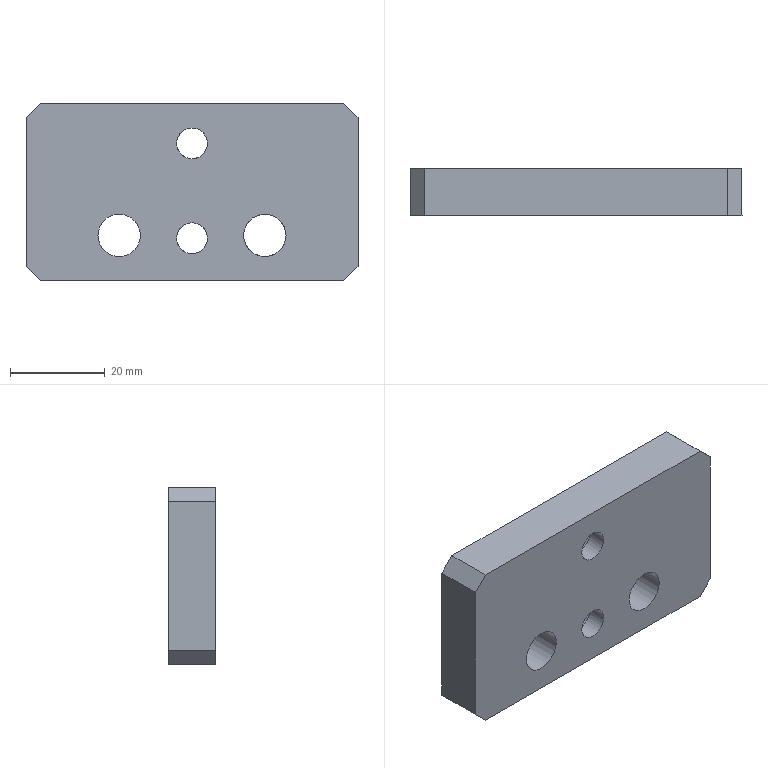Part | STEP file | 1_id1138_x_t | 1 solid | 18 faces | box 70 x 10 x 37.5 mm | volume 23507 mm3 | plane 12 | cylinder 6 | commonest cylinder face diameters 6.5 x2 8.95 x2 10.5 x2
STEP:
#1=CARTESIAN_POINT('',(0.,0.,0.));
#2=DIRECTION('',(0.,0.,1.));
#3=DIRECTION('',(1.,0.,0.));
#4=AXIS2_PLACEMENT_3D('',#1,#2,#3);
#5=CARTESIAN_POINT('',(750.075,188.975,-66.026));
#6=VERTEX_POINT('',#5);
#7=CARTESIAN_POINT('',(750.075,188.975,-71.276));
#8=DIRECTION('',(0.,1.,0.));
#9=DIRECTION('',(0.,0.,1.));
#10=AXIS2_PLACEMENT_3D('',#7,#8,#9);
#11=CIRCLE('',#10,5.25);
#12=CARTESIAN_POINT('',(750.075,188.975,-71.276));
#13=DIRECTION('',(0.,-1.,0.));
#14=DIRECTION('',(0.,0.,1.));
#15=AXIS2_PLACEMENT_3D('',#12,#13,#14);
#16=PLANE('',#15);
#17=CARTESIAN_POINT('',(5.25,0.));
#18=CARTESIAN_POINT('',(5.25,-9.093));
#19=CARTESIAN_POINT('',(-2.625,-4.547));
#20=CARTESIAN_POINT('',(-10.5,0.));
#21=CARTESIAN_POINT('',(-2.625,4.547));
#22=CARTESIAN_POINT('',(5.25,9.093));
#23=CARTESIAN_POINT('',(5.25,0.));
#24=(BOUNDED_CURVE()B_SPLINE_CURVE(2,(#17,#18,#19,#20,#21,#22,#23),.UNSPECIFIED.,.T.,.F.)B_SPLINE_CURVE_WITH_KNOTS((1,2,2,2,2,1),(-2.094,0.,2.094,4.189,6.283,8.378),.UNSPECIFIED.)CURVE()GEOMETRIC_REPRESENTATION_ITEM()RATIONAL_B_SPLINE_CURVE((1.,0.5,1.,0.5,1.,0.5,1.))REPRESENTATION_ITEM(''));
#25=(GEOMETRIC_REPRESENTATION_CONTEXT(2)PARAMETRIC_REPRESENTATION_CONTEXT()REPRESENTATION_CONTEXT('',''));
#26=DEFINITIONAL_REPRESENTATION('',(#24),#25);
#27=PCURVE('',#16,#26);
#28=CARTESIAN_POINT('',(750.075,194.975,-71.276));
#29=DIRECTION('',(0.,-1.,0.));
#30=DIRECTION('',(0.,0.,1.));
#31=AXIS2_PLACEMENT_3D('',#28,#29,#30);
#32=CYLINDRICAL_SURFACE('',#31,5.25);
#33=CARTESIAN_POINT('',(6.283,6.));
#34=DIRECTION('',(-1.,0.));
#35=VECTOR('',#34,1.);
#36=LINE('',#33,#35);
#37=(GEOMETRIC_REPRESENTATION_CONTEXT(2)PARAMETRIC_REPRESENTATION_CONTEXT()REPRESENTATION_CONTEXT('',''));
#38=DEFINITIONAL_REPRESENTATION('',(#36),#37);
#39=PCURVE('',#32,#38);
#40=SURFACE_CURVE('',#11,(#27,#39),.PCURVE_S1.);
#41=EDGE_CURVE('',#6,#6,#40,.T.);
#42=ORIENTED_EDGE('',*,*,#41,.T.);
#43=EDGE_LOOP('',(#42));
#44=FACE_BOUND('',#43,.T.);
#45=CARTESIAN_POINT('',(750.075,188.975,-74.526));
#46=VERTEX_POINT('',#45);
#47=CARTESIAN_POINT('',(750.075,188.975,-71.276));
#48=DIRECTION('',(0.,-1.,0.));
#49=DIRECTION('',(0.,0.,-1.));
#50=AXIS2_PLACEMENT_3D('',#47,#48,#49);
#51=CIRCLE('',#50,3.25);
#52=CARTESIAN_POINT('',(0.,-0.000000001));
#53=DIRECTION('',(-1.,0.));
#54=AXIS2_PLACEMENT_2D('',#52,#53);
#55=CIRCLE('',#54,3.25);
#56=(GEOMETRIC_REPRESENTATION_CONTEXT(2)PARAMETRIC_REPRESENTATION_CONTEXT()REPRESENTATION_CONTEXT('',''));
#57=DEFINITIONAL_REPRESENTATION('',(#55),#56);
#58=PCURVE('',#16,#57);
#59=CARTESIAN_POINT('',(750.075,185.725,-71.276));
#60=DIRECTION('',(0.,-1.,0.));
#61=DIRECTION('',(-1.,0.,0.));
#62=AXIS2_PLACEMENT_3D('',#59,#60,#61);
#63=CYLINDRICAL_SURFACE('',#62,3.25);
#64=CARTESIAN_POINT('',(1.571,-3.25));
#65=DIRECTION('',(1.,0.));
#66=VECTOR('',#65,1.);
#67=LINE('',#64,#66);
#68=(GEOMETRIC_REPRESENTATION_CONTEXT(2)PARAMETRIC_REPRESENTATION_CONTEXT()REPRESENTATION_CONTEXT('',''));
#69=DEFINITIONAL_REPRESENTATION('',(#67),#68);
#70=PCURVE('',#63,#69);
#71=SURFACE_CURVE('',#51,(#58,#70),.PCURVE_S1.);
#72=EDGE_CURVE('',#46,#46,#71,.T.);
#73=ORIENTED_EDGE('',*,*,#72,.T.);
#74=EDGE_LOOP('',(#73));
#75=FACE_BOUND('',#74,.T.);
#76=ADVANCED_FACE('',(#44,#75),#16,.F.);
#77=ORIENTED_EDGE('',*,*,#41,.T.);
#78=CARTESIAN_POINT('',(750.075,194.975,-66.026));
#79=VERTEX_POINT('',#78);
#80=CARTESIAN_POINT('',(750.075,194.975,-66.026));
#81=CARTESIAN_POINT('',(750.075,188.975,-66.026));
#82=B_SPLINE_CURVE_WITH_KNOTS('',1,(#80,#81),.UNSPECIFIED.,.F.,.F.,(2,2),(-0.000000002,6.),.PIECEWISE_BEZIER_KNOTS.);
#83=CARTESIAN_POINT('',(0.,0.));
#84=DIRECTION('',(0.,1.));
#85=VECTOR('',#84,1.);
#86=LINE('',#83,#85);
#87=(GEOMETRIC_REPRESENTATION_CONTEXT(2)PARAMETRIC_REPRESENTATION_CONTEXT()REPRESENTATION_CONTEXT('',''));
#88=DEFINITIONAL_REPRESENTATION('',(#86),#87);
#89=PCURVE('',#32,#88);
#90=CARTESIAN_POINT('',(6.283,0.));
#91=DIRECTION('',(0.,1.));
#92=VECTOR('',#91,1.);
#93=LINE('',#90,#92);
#94=(GEOMETRIC_REPRESENTATION_CONTEXT(2)PARAMETRIC_REPRESENTATION_CONTEXT()REPRESENTATION_CONTEXT('',''));
#95=DEFINITIONAL_REPRESENTATION('',(#93),#94);
#96=PCURVE('',#32,#95);
#97=SEAM_CURVE('',#82,(#89,#96),.PCURVE_S1.);
#98=EDGE_CURVE('',#79,#6,#97,.T.);
#99=ORIENTED_EDGE('',*,*,#98,.F.);
#100=CARTESIAN_POINT('',(750.075,194.975,-76.526));
#101=VERTEX_POINT('',#100);
#102=CARTESIAN_POINT('',(750.075,194.975,-71.276));
#103=DIRECTION('',(0.,-1.,0.));
#104=DIRECTION('',(0.,0.,-1.));
#105=AXIS2_PLACEMENT_3D('',#102,#103,#104);
#106=CIRCLE('',#105,5.25);
#107=CARTESIAN_POINT('',(-3.142,-0.000000002));
#108=DIRECTION('',(1.,0.));
#109=VECTOR('',#108,1.);
#110=LINE('',#107,#109);
#111=(GEOMETRIC_REPRESENTATION_CONTEXT(2)PARAMETRIC_REPRESENTATION_CONTEXT()REPRESENTATION_CONTEXT('',''));
#112=DEFINITIONAL_REPRESENTATION('',(#110),#111);
#113=PCURVE('',#32,#112);
#114=CARTESIAN_POINT('',(784.423,194.975,-37.776));
#115=DIRECTION('',(0.,1.,0.));
#116=DIRECTION('',(1.,0.,0.));
#117=AXIS2_PLACEMENT_3D('',#114,#115,#116);
#118=PLANE('',#117);
#119=CARTESIAN_POINT('',(-34.348,38.75));
#120=CARTESIAN_POINT('',(-25.254,38.75));
#121=CARTESIAN_POINT('',(-29.801,30.875));
#122=CARTESIAN_POINT('',(-34.348,23.));
#123=CARTESIAN_POINT('',(-38.894,30.875));
#124=CARTESIAN_POINT('',(-43.441,38.75));
#125=CARTESIAN_POINT('',(-34.348,38.75));
#126=(BOUNDED_CURVE()B_SPLINE_CURVE(2,(#119,#120,#121,#122,#123,#124,#125),.UNSPECIFIED.,.T.,.F.)B_SPLINE_CURVE_WITH_KNOTS((1,2,2,2,2,1),(-2.094,0.,2.094,4.189,6.283,8.378),.UNSPECIFIED.)CURVE()GEOMETRIC_REPRESENTATION_ITEM()RATIONAL_B_SPLINE_CURVE((1.,0.5,1.,0.5,1.,0.5,1.))REPRESENTATION_ITEM(''));
#127=(GEOMETRIC_REPRESENTATION_CONTEXT(2)PARAMETRIC_REPRESENTATION_CONTEXT()REPRESENTATION_CONTEXT('',''));
#128=DEFINITIONAL_REPRESENTATION('',(#126),#127);
#129=PCURVE('',#118,#128);
#130=SURFACE_CURVE('',#106,(#113,#129),.PCURVE_S1.);
#131=EDGE_CURVE('',#79,#101,#130,.T.);
#132=ORIENTED_EDGE('',*,*,#131,.T.);
#133=CARTESIAN_POINT('',(750.075,194.975,-71.276));
#134=DIRECTION('',(0.,-1.,0.));
#135=DIRECTION('',(0.,0.,-1.));
#136=AXIS2_PLACEMENT_3D('',#133,#134,#135);
#137=CIRCLE('',#136,5.25);
#138=CARTESIAN_POINT('',(3.142,-0.000000002));
#139=DIRECTION('',(1.,0.));
#140=VECTOR('',#139,1.);
#141=LINE('',#138,#140);
#142=(GEOMETRIC_REPRESENTATION_CONTEXT(2)PARAMETRIC_REPRESENTATION_CONTEXT()REPRESENTATION_CONTEXT('',''));
#143=DEFINITIONAL_REPRESENTATION('',(#141),#142);
#144=PCURVE('',#32,#143);
#145=CARTESIAN_POINT('',(-34.348,38.75));
#146=CARTESIAN_POINT('',(-25.254,38.75));
#147=CARTESIAN_POINT('',(-29.801,30.875));
#148=CARTESIAN_POINT('',(-34.348,23.));
#149=CARTESIAN_POINT('',(-38.894,30.875));
#150=CARTESIAN_POINT('',(-43.441,38.75));
#151=CARTESIAN_POINT('',(-34.348,38.75));
#152=(BOUNDED_CURVE()B_SPLINE_CURVE(2,(#145,#146,#147,#148,#149,#150,#151),.UNSPECIFIED.,.T.,.F.)B_SPLINE_CURVE_WITH_KNOTS((1,2,2,2,2,1),(-2.094,0.,2.094,4.189,6.283,8.378),.UNSPECIFIED.)CURVE()GEOMETRIC_REPRESENTATION_ITEM()RATIONAL_B_SPLINE_CURVE((1.,0.5,1.,0.5,1.,0.5,1.))REPRESENTATION_ITEM(''));
#153=(GEOMETRIC_REPRESENTATION_CONTEXT(2)PARAMETRIC_REPRESENTATION_CONTEXT()REPRESENTATION_CONTEXT('',''));
#154=DEFINITIONAL_REPRESENTATION('',(#152),#153);
#155=PCURVE('',#118,#154);
#156=SURFACE_CURVE('',#137,(#144,#155),.PCURVE_S1.);
#157=EDGE_CURVE('',#101,#79,#156,.T.);
#158=ORIENTED_EDGE('',*,*,#157,.T.);
#159=ORIENTED_EDGE('',*,*,#98,.T.);
#160=EDGE_LOOP('',(#77,#99,#132,#158,#159));
#161=FACE_BOUND('',#160,.F.);
#162=ADVANCED_FACE('',(#161),#32,.F.);
#163=CARTESIAN_POINT('',(785.075,194.975,-77.276));
#164=VERTEX_POINT('',#163);
#165=CARTESIAN_POINT('',(782.075,194.975,-80.276));
#166=VERTEX_POINT('',#165);
#167=CARTESIAN_POINT('',(785.075,194.975,-77.276));
#168=DIRECTION('',(-0.7071,0.,-0.7071));
#169=VECTOR('',#168,1.);
#170=LINE('',#167,#169);
#171=CARTESIAN_POINT('',(0.6524,39.5));
#172=DIRECTION('',(-0.7071,0.7071));
#173=VECTOR('',#172,1.);
#174=LINE('',#171,#173);
#175=(GEOMETRIC_REPRESENTATION_CONTEXT(2)PARAMETRIC_REPRESENTATION_CONTEXT()REPRESENTATION_CONTEXT('',''));
#176=DEFINITIONAL_REPRESENTATION('',(#174),#175);
#177=PCURVE('',#118,#176);
#178=CARTESIAN_POINT('',(782.075,183.425,-80.276));
#179=DIRECTION('',(-0.7071,0.,0.7071));
#180=DIRECTION('',(0.7071,0.,0.7071));
#181=AXIS2_PLACEMENT_3D('',#178,#179,#180);
#182=PLANE('',#181);
#183=CARTESIAN_POINT('',(4.243,11.55));
#184=DIRECTION('',(-1.,0.));
#185=VECTOR('',#184,1.);
#186=LINE('',#183,#185);
#187=(GEOMETRIC_REPRESENTATION_CONTEXT(2)PARAMETRIC_REPRESENTATION_CONTEXT()REPRESENTATION_CONTEXT('',''));
#188=DEFINITIONAL_REPRESENTATION('',(#186),#187);
#189=PCURVE('',#182,#188);
#190=SURFACE_CURVE('',#170,(#177,#189),.PCURVE_S1.);
#191=EDGE_CURVE('',#164,#166,#190,.T.);
#192=ORIENTED_EDGE('',*,*,#191,.T.);
#193=CARTESIAN_POINT('',(718.075,194.975,-80.276));
#194=VERTEX_POINT('',#193);
#195=CARTESIAN_POINT('',(718.075,194.975,-80.276));
#196=DIRECTION('',(1.,0.,0.));
#197=VECTOR('',#196,1.);
#198=LINE('',#195,#197);
#199=CARTESIAN_POINT('',(-66.348,42.5));
#200=DIRECTION('',(1.,0.));
#201=VECTOR('',#200,1.);
#202=LINE('',#199,#201);
#203=(GEOMETRIC_REPRESENTATION_CONTEXT(2)PARAMETRIC_REPRESENTATION_CONTEXT()REPRESENTATION_CONTEXT('',''));
#204=DEFINITIONAL_REPRESENTATION('',(#202),#203);
#205=PCURVE('',#118,#204);
#206=CARTESIAN_POINT('',(728.423,183.425,-80.276));
#207=DIRECTION('',(0.,0.,1.));
#208=DIRECTION('',(-1.,0.,0.));
#209=AXIS2_PLACEMENT_3D('',#206,#207,#208);
#210=PLANE('',#209);
#211=CARTESIAN_POINT('',(10.348,-11.55));
#212=DIRECTION('',(-1.,0.));
#213=VECTOR('',#212,1.);
#214=LINE('',#211,#213);
#215=(GEOMETRIC_REPRESENTATION_CONTEXT(2)PARAMETRIC_REPRESENTATION_CONTEXT()REPRESENTATION_CONTEXT('',''));
#216=DEFINITIONAL_REPRESENTATION('',(#214),#215);
#217=PCURVE('',#210,#216);
#218=SURFACE_CURVE('',#198,(#205,#217),.PCURVE_S1.);
#219=EDGE_CURVE('',#194,#166,#218,.T.);
#220=ORIENTED_EDGE('',*,*,#219,.F.);
#221=CARTESIAN_POINT('',(715.075,194.975,-77.276));
#222=VERTEX_POINT('',#221);
#223=CARTESIAN_POINT('',(718.075,194.975,-80.276));
#224=DIRECTION('',(-0.7071,0.,0.7071));
#225=VECTOR('',#224,1.);
#226=LINE('',#223,#225);
#227=CARTESIAN_POINT('',(-66.348,42.5));
#228=DIRECTION('',(-0.7071,-0.7071));
#229=VECTOR('',#228,1.);
#230=LINE('',#227,#229);
#231=(GEOMETRIC_REPRESENTATION_CONTEXT(2)PARAMETRIC_REPRESENTATION_CONTEXT()REPRESENTATION_CONTEXT('',''));
#232=DEFINITIONAL_REPRESENTATION('',(#230),#231);
#233=PCURVE('',#118,#232);
#234=CARTESIAN_POINT('',(718.075,183.425,-80.276));
#235=DIRECTION('',(0.7071,0.,0.7071));
#236=DIRECTION('',(0.7071,0.,-0.7071));
#237=AXIS2_PLACEMENT_3D('',#234,#235,#236);
#238=PLANE('',#237);
#239=CARTESIAN_POINT('',(0.,11.55));
#240=DIRECTION('',(-1.,0.));
#241=VECTOR('',#240,1.);
#242=LINE('',#239,#241);
#243=(GEOMETRIC_REPRESENTATION_CONTEXT(2)PARAMETRIC_REPRESENTATION_CONTEXT()REPRESENTATION_CONTEXT('',''));
#244=DEFINITIONAL_REPRESENTATION('',(#242),#243);
#245=PCURVE('',#238,#244);
#246=SURFACE_CURVE('',#226,(#233,#245),.PCURVE_S1.);
#247=EDGE_CURVE('',#194,#222,#246,.T.);
#248=ORIENTED_EDGE('',*,*,#247,.T.);
#249=CARTESIAN_POINT('',(715.075,194.975,-45.776));
#250=VERTEX_POINT('',#249);
#251=CARTESIAN_POINT('',(715.075,194.975,-77.276));
#252=DIRECTION('',(0.,0.,1.));
#253=VECTOR('',#252,1.);
#254=LINE('',#251,#253);
#255=CARTESIAN_POINT('',(-69.348,39.5));
#256=DIRECTION('',(0.,-1.));
#257=VECTOR('',#256,1.);
#258=LINE('',#255,#257);
#259=(GEOMETRIC_REPRESENTATION_CONTEXT(2)PARAMETRIC_REPRESENTATION_CONTEXT()REPRESENTATION_CONTEXT('',''));
#260=DEFINITIONAL_REPRESENTATION('',(#258),#259);
#261=PCURVE('',#118,#260);
#262=CARTESIAN_POINT('',(715.075,191.975,-61.526));
#263=DIRECTION('',(1.,0.,0.));
#264=DIRECTION('',(0.,0.,-1.));
#265=AXIS2_PLACEMENT_3D('',#262,#263,#264);
#266=PLANE('',#265);
#267=CARTESIAN_POINT('',(15.75,3.));
#268=DIRECTION('',(-1.,0.));
#269=VECTOR('',#268,1.);
#270=LINE('',#267,#269);
#271=(GEOMETRIC_REPRESENTATION_CONTEXT(2)PARAMETRIC_REPRESENTATION_CONTEXT()REPRESENTATION_CONTEXT('',''));
#272=DEFINITIONAL_REPRESENTATION('',(#270),#271);
#273=PCURVE('',#266,#272);
#274=SURFACE_CURVE('',#254,(#261,#273),.PCURVE_S1.);
#275=EDGE_CURVE('',#222,#250,#274,.T.);
#276=ORIENTED_EDGE('',*,*,#275,.T.);
#277=CARTESIAN_POINT('',(718.075,194.975,-42.776));
#278=VERTEX_POINT('',#277);
#279=CARTESIAN_POINT('',(715.075,194.975,-45.776));
#280=DIRECTION('',(0.7071,0.,0.7071));
#281=VECTOR('',#280,1.);
#282=LINE('',#279,#281);
#283=CARTESIAN_POINT('',(-69.348,8.));
#284=DIRECTION('',(0.7071,-0.7071));
#285=VECTOR('',#284,1.);
#286=LINE('',#283,#285);
#287=(GEOMETRIC_REPRESENTATION_CONTEXT(2)PARAMETRIC_REPRESENTATION_CONTEXT()REPRESENTATION_CONTEXT('',''));
#288=DEFINITIONAL_REPRESENTATION('',(#286),#287);
#289=PCURVE('',#118,#288);
#290=CARTESIAN_POINT('',(718.075,183.425,-42.776));
#291=DIRECTION('',(0.7071,0.,-0.7071));
#292=DIRECTION('',(-0.7071,0.,-0.7071));
#293=AXIS2_PLACEMENT_3D('',#290,#291,#292);
#294=PLANE('',#293);
#295=CARTESIAN_POINT('',(4.243,11.55));
#296=DIRECTION('',(-1.,0.));
#297=VECTOR('',#296,1.);
#298=LINE('',#295,#297);
#299=(GEOMETRIC_REPRESENTATION_CONTEXT(2)PARAMETRIC_REPRESENTATION_CONTEXT()REPRESENTATION_CONTEXT('',''));
#300=DEFINITIONAL_REPRESENTATION('',(#298),#299);
#301=PCURVE('',#294,#300);
#302=SURFACE_CURVE('',#282,(#289,#301),.PCURVE_S1.);
#303=EDGE_CURVE('',#250,#278,#302,.T.);
#304=ORIENTED_EDGE('',*,*,#303,.T.);
#305=CARTESIAN_POINT('',(782.075,194.975,-42.776));
#306=VERTEX_POINT('',#305);
#307=CARTESIAN_POINT('',(782.075,194.975,-42.776));
#308=DIRECTION('',(-1.,0.,0.));
#309=VECTOR('',#308,1.);
#310=LINE('',#307,#309);
#311=CARTESIAN_POINT('',(-2.348,5.));
#312=DIRECTION('',(-1.,0.));
#313=VECTOR('',#312,1.);
#314=LINE('',#311,#313);
#315=(GEOMETRIC_REPRESENTATION_CONTEXT(2)PARAMETRIC_REPRESENTATION_CONTEXT()REPRESENTATION_CONTEXT('',''));
#316=DEFINITIONAL_REPRESENTATION('',(#314),#315);
#317=PCURVE('',#118,#316);
#318=CARTESIAN_POINT('',(775.423,183.425,-42.776));
#319=DIRECTION('',(0.,0.,-1.));
#320=DIRECTION('',(0.,-1.,0.));
#321=AXIS2_PLACEMENT_3D('',#318,#319,#320);
#322=PLANE('',#321);
#323=CARTESIAN_POINT('',(-11.55,-6.652));
#324=DIRECTION('',(0.,1.));
#325=VECTOR('',#324,1.);
#326=LINE('',#323,#325);
#327=(GEOMETRIC_REPRESENTATION_CONTEXT(2)PARAMETRIC_REPRESENTATION_CONTEXT()REPRESENTATION_CONTEXT('',''));
#328=DEFINITIONAL_REPRESENTATION('',(#326),#327);
#329=PCURVE('',#322,#328);
#330=SURFACE_CURVE('',#310,(#317,#329),.PCURVE_S1.);
#331=EDGE_CURVE('',#306,#278,#330,.T.);
#332=ORIENTED_EDGE('',*,*,#331,.F.);
#333=CARTESIAN_POINT('',(785.075,194.975,-45.776));
#334=VERTEX_POINT('',#333);
#335=CARTESIAN_POINT('',(782.075,194.975,-42.776));
#336=DIRECTION('',(0.7071,0.,-0.7071));
#337=VECTOR('',#336,1.);
#338=LINE('',#335,#337);
#339=CARTESIAN_POINT('',(-2.348,5.));
#340=DIRECTION('',(0.7071,0.7071));
#341=VECTOR('',#340,1.);
#342=LINE('',#339,#341);
#343=(GEOMETRIC_REPRESENTATION_CONTEXT(2)PARAMETRIC_REPRESENTATION_CONTEXT()REPRESENTATION_CONTEXT('',''));
#344=DEFINITIONAL_REPRESENTATION('',(#342),#343);
#345=PCURVE('',#118,#344);
#346=CARTESIAN_POINT('',(782.075,183.425,-42.776));
#347=DIRECTION('',(-0.7071,0.,-0.7071));
#348=DIRECTION('',(-0.7071,0.,0.7071));
#349=AXIS2_PLACEMENT_3D('',#346,#347,#348);
#350=PLANE('',#349);
#351=CARTESIAN_POINT('',(0.,11.55));
#352=DIRECTION('',(-1.,0.));
#353=VECTOR('',#352,1.);
#354=LINE('',#351,#353);
#355=(GEOMETRIC_REPRESENTATION_CONTEXT(2)PARAMETRIC_REPRESENTATION_CONTEXT()REPRESENTATION_CONTEXT('',''));
#356=DEFINITIONAL_REPRESENTATION('',(#354),#355);
#357=PCURVE('',#350,#356);
#358=SURFACE_CURVE('',#338,(#345,#357),.PCURVE_S1.);
#359=EDGE_CURVE('',#306,#334,#358,.T.);
#360=ORIENTED_EDGE('',*,*,#359,.T.);
#361=CARTESIAN_POINT('',(785.075,194.975,-45.776));
#362=DIRECTION('',(0.,0.,-1.));
#363=VECTOR('',#362,1.);
#364=LINE('',#361,#363);
#365=CARTESIAN_POINT('',(0.6524,8.));
#366=DIRECTION('',(0.,1.));
#367=VECTOR('',#366,1.);
#368=LINE('',#365,#367);
#369=(GEOMETRIC_REPRESENTATION_CONTEXT(2)PARAMETRIC_REPRESENTATION_CONTEXT()REPRESENTATION_CONTEXT('',''));
#370=DEFINITIONAL_REPRESENTATION('',(#368),#369);
#371=PCURVE('',#118,#370);
#372=CARTESIAN_POINT('',(785.075,191.975,-57.036));
#373=DIRECTION('',(-1.,0.,0.));
#374=DIRECTION('',(0.,-1.,0.));
#375=AXIS2_PLACEMENT_3D('',#372,#373,#374);
#376=PLANE('',#375);
#377=CARTESIAN_POINT('',(-3.,11.26));
#378=DIRECTION('',(0.,-1.));
#379=VECTOR('',#378,1.);
#380=LINE('',#377,#379);
#381=(GEOMETRIC_REPRESENTATION_CONTEXT(2)PARAMETRIC_REPRESENTATION_CONTEXT()REPRESENTATION_CONTEXT('',''));
#382=DEFINITIONAL_REPRESENTATION('',(#380),#381);
#383=PCURVE('',#376,#382);
#384=SURFACE_CURVE('',#364,(#371,#383),.PCURVE_S1.);
#385=EDGE_CURVE('',#334,#164,#384,.T.);
#386=ORIENTED_EDGE('',*,*,#385,.T.);
#387=EDGE_LOOP('',(#192,#220,#248,#276,#304,#332,#360,#386));
#388=FACE_BOUND('',#387,.T.);
#389=CARTESIAN_POINT('',(744.825,194.975,-51.276));
#390=VERTEX_POINT('',#389);
#391=CARTESIAN_POINT('',(750.075,194.975,-51.276));
#392=DIRECTION('',(0.,-1.,0.));
#393=DIRECTION('',(-1.,0.,0.));
#394=AXIS2_PLACEMENT_3D('',#391,#392,#393);
#395=CIRCLE('',#394,5.25);
#396=CARTESIAN_POINT('',(-39.598,13.5));
#397=CARTESIAN_POINT('',(-39.598,22.593));
#398=CARTESIAN_POINT('',(-31.723,18.047));
#399=CARTESIAN_POINT('',(-23.848,13.5));
#400=CARTESIAN_POINT('',(-31.723,8.953));
#401=CARTESIAN_POINT('',(-39.598,4.407));
#402=CARTESIAN_POINT('',(-39.598,13.5));
#403=(BOUNDED_CURVE()B_SPLINE_CURVE(2,(#396,#397,#398,#399,#400,#401,#402),.UNSPECIFIED.,.T.,.F.)B_SPLINE_CURVE_WITH_KNOTS((1,2,2,2,2,1),(-2.094,0.,2.094,4.189,6.283,8.378),.UNSPECIFIED.)CURVE()GEOMETRIC_REPRESENTATION_ITEM()RATIONAL_B_SPLINE_CURVE((1.,0.5,1.,0.5,1.,0.5,1.))REPRESENTATION_ITEM(''));
#404=(GEOMETRIC_REPRESENTATION_CONTEXT(2)PARAMETRIC_REPRESENTATION_CONTEXT()REPRESENTATION_CONTEXT('',''));
#405=DEFINITIONAL_REPRESENTATION('',(#403),#404);
#406=PCURVE('',#118,#405);
#407=CARTESIAN_POINT('',(750.075,194.975,-51.276));
#408=DIRECTION('',(0.,-1.,0.));
#409=DIRECTION('',(0.,0.,1.));
#410=AXIS2_PLACEMENT_3D('',#407,#408,#409);
#411=CYLINDRICAL_SURFACE('',#410,5.25);
#412=CARTESIAN_POINT('',(1.571,0.000000001));
#413=DIRECTION('',(1.,0.));
#414=VECTOR('',#413,1.);
#415=LINE('',#412,#414);
#416=(GEOMETRIC_REPRESENTATION_CONTEXT(2)PARAMETRIC_REPRESENTATION_CONTEXT()REPRESENTATION_CONTEXT('',''));
#417=DEFINITIONAL_REPRESENTATION('',(#415),#416);
#418=PCURVE('',#411,#417);
#419=SURFACE_CURVE('',#395,(#406,#418),.PCURVE_S1.);
#420=EDGE_CURVE('',#390,#390,#419,.T.);
#421=ORIENTED_EDGE('',*,*,#420,.T.);
#422=EDGE_LOOP('',(#421));
#423=FACE_BOUND('',#422,.T.);
#424=ORIENTED_EDGE('',*,*,#157,.T.);
#425=ORIENTED_EDGE('',*,*,#131,.T.);
#426=EDGE_LOOP('',(#424,#425));
#427=FACE_BOUND('',#426,.T.);
#428=CARTESIAN_POINT('',(730.25,194.975,-70.67));
#429=VERTEX_POINT('',#428);
#430=CARTESIAN_POINT('',(734.725,194.975,-70.67));
#431=DIRECTION('',(0.,-1.,0.));
#432=DIRECTION('',(-1.,0.,0.));
#433=AXIS2_PLACEMENT_3D('',#430,#431,#432);
#434=CIRCLE('',#433,4.475);
#435=CARTESIAN_POINT('',(-54.173,32.894));
#436=CARTESIAN_POINT('',(-54.173,40.645));
#437=CARTESIAN_POINT('',(-47.46,36.769));
#438=CARTESIAN_POINT('',(-40.748,32.894));
#439=CARTESIAN_POINT('',(-47.46,29.019));
#440=CARTESIAN_POINT('',(-54.173,25.143));
#441=CARTESIAN_POINT('',(-54.173,32.894));
#442=(BOUNDED_CURVE()B_SPLINE_CURVE(2,(#435,#436,#437,#438,#439,#440,#441),.UNSPECIFIED.,.T.,.F.)B_SPLINE_CURVE_WITH_KNOTS((1,2,2,2,2,1),(-2.094,0.,2.094,4.189,6.283,8.378),.UNSPECIFIED.)CURVE()GEOMETRIC_REPRESENTATION_ITEM()RATIONAL_B_SPLINE_CURVE((1.,0.5,1.,0.5,1.,0.5,1.))REPRESENTATION_ITEM(''));
#443=(GEOMETRIC_REPRESENTATION_CONTEXT(2)PARAMETRIC_REPRESENTATION_CONTEXT()REPRESENTATION_CONTEXT('',''));
#444=DEFINITIONAL_REPRESENTATION('',(#442),#443);
#445=PCURVE('',#118,#444);
#446=CARTESIAN_POINT('',(734.725,124.975,-70.67));
#447=DIRECTION('',(0.,1.,0.));
#448=DIRECTION('',(-1.,0.,0.));
#449=AXIS2_PLACEMENT_3D('',#446,#447,#448);
#450=CYLINDRICAL_SURFACE('',#449,4.475);
#451=CARTESIAN_POINT('',(6.283,70.));
#452=DIRECTION('',(-1.,0.));
#453=VECTOR('',#452,1.);
#454=LINE('',#451,#453);
#455=(GEOMETRIC_REPRESENTATION_CONTEXT(2)PARAMETRIC_REPRESENTATION_CONTEXT()REPRESENTATION_CONTEXT('',''));
#456=DEFINITIONAL_REPRESENTATION('',(#454),#455);
#457=PCURVE('',#450,#456);
#458=SURFACE_CURVE('',#434,(#445,#457),.PCURVE_S1.);
#459=EDGE_CURVE('',#429,#429,#458,.T.);
#460=ORIENTED_EDGE('',*,*,#459,.T.);
#461=EDGE_LOOP('',(#460));
#462=FACE_BOUND('',#461,.T.);
#463=CARTESIAN_POINT('',(765.425,194.975,-75.145));
#464=VERTEX_POINT('',#463);
#465=CARTESIAN_POINT('',(769.9,194.975,-70.67));
#466=VERTEX_POINT('',#465);
#467=CARTESIAN_POINT('',(765.425,194.975,-70.67));
#468=DIRECTION('',(0.,-1.,0.));
#469=DIRECTION('',(0.,0.,-1.));
#470=AXIS2_PLACEMENT_3D('',#467,#468,#469);
#471=CIRCLE('',#470,4.475);
#472=CARTESIAN_POINT('',(-18.998,37.369));
#473=CARTESIAN_POINT('',(-11.247,37.369));
#474=CARTESIAN_POINT('',(-15.122,30.657));
#475=CARTESIAN_POINT('',(-18.998,23.944));
#476=CARTESIAN_POINT('',(-22.873,30.657));
#477=CARTESIAN_POINT('',(-26.749,37.369));
#478=CARTESIAN_POINT('',(-18.998,37.369));
#479=(BOUNDED_CURVE()B_SPLINE_CURVE(2,(#472,#473,#474,#475,#476,#477,#478),.UNSPECIFIED.,.T.,.F.)B_SPLINE_CURVE_WITH_KNOTS((1,2,2,2,2,1),(-2.094,0.,2.094,4.189,6.283,8.378),.UNSPECIFIED.)CURVE()GEOMETRIC_REPRESENTATION_ITEM()RATIONAL_B_SPLINE_CURVE((1.,0.5,1.,0.5,1.,0.5,1.))REPRESENTATION_ITEM(''));
#480=(GEOMETRIC_REPRESENTATION_CONTEXT(2)PARAMETRIC_REPRESENTATION_CONTEXT()REPRESENTATION_CONTEXT('',''));
#481=DEFINITIONAL_REPRESENTATION('',(#479),#480);
#482=PCURVE('',#118,#481);
#483=CARTESIAN_POINT('',(765.425,186.235,-70.67));
#484=DIRECTION('',(0.,-1.,0.));
#485=DIRECTION('',(0.,0.,1.));
#486=AXIS2_PLACEMENT_3D('',#483,#484,#485);
#487=CYLINDRICAL_SURFACE('',#486,4.475);
#488=CARTESIAN_POINT('',(9.425,-8.74));
#489=DIRECTION('',(1.,0.));
#490=VECTOR('',#489,1.);
#491=LINE('',#488,#490);
#492=(GEOMETRIC_REPRESENTATION_CONTEXT(2)PARAMETRIC_REPRESENTATION_CONTEXT()REPRESENTATION_CONTEXT('',''));
#493=DEFINITIONAL_REPRESENTATION('',(#491),#492);
#494=PCURVE('',#487,#493);
#495=SURFACE_CURVE('',#471,(#482,#494),.PCURVE_S1.);
#496=EDGE_CURVE('',#464,#466,#495,.T.);
#497=ORIENTED_EDGE('',*,*,#496,.T.);
#498=CARTESIAN_POINT('',(765.425,194.975,-70.67));
#499=DIRECTION('',(0.,-1.,0.));
#500=DIRECTION('',(0.,0.,-1.));
#501=AXIS2_PLACEMENT_3D('',#498,#499,#500);
#502=CIRCLE('',#501,4.475);
#503=CARTESIAN_POINT('',(-18.998,37.369));
#504=CARTESIAN_POINT('',(-11.247,37.369));
#505=CARTESIAN_POINT('',(-15.122,30.657));
#506=CARTESIAN_POINT('',(-18.998,23.944));
#507=CARTESIAN_POINT('',(-22.873,30.657));
#508=CARTESIAN_POINT('',(-26.749,37.369));
#509=CARTESIAN_POINT('',(-18.998,37.369));
#510=(BOUNDED_CURVE()B_SPLINE_CURVE(2,(#503,#504,#505,#506,#507,#508,#509),.UNSPECIFIED.,.T.,.F.)B_SPLINE_CURVE_WITH_KNOTS((1,2,2,2,2,1),(-2.094,0.,2.094,4.189,6.283,8.378),.UNSPECIFIED.)CURVE()GEOMETRIC_REPRESENTATION_ITEM()RATIONAL_B_SPLINE_CURVE((1.,0.5,1.,0.5,1.,0.5,1.))REPRESENTATION_ITEM(''));
#511=(GEOMETRIC_REPRESENTATION_CONTEXT(2)PARAMETRIC_REPRESENTATION_CONTEXT()REPRESENTATION_CONTEXT('',''));
#512=DEFINITIONAL_REPRESENTATION('',(#510),#511);
#513=PCURVE('',#118,#512);
#514=CARTESIAN_POINT('',(3.142,-8.74));
#515=DIRECTION('',(1.,0.));
#516=VECTOR('',#515,1.);
#517=LINE('',#514,#516);
#518=(GEOMETRIC_REPRESENTATION_CONTEXT(2)PARAMETRIC_REPRESENTATION_CONTEXT()REPRESENTATION_CONTEXT('',''));
#519=DEFINITIONAL_REPRESENTATION('',(#517),#518);
#520=PCURVE('',#487,#519);
#521=SURFACE_CURVE('',#502,(#513,#520),.PCURVE_S1.);
#522=EDGE_CURVE('',#466,#464,#521,.T.);
#523=ORIENTED_EDGE('',*,*,#522,.T.);
#524=EDGE_LOOP('',(#497,#523));
#525=FACE_BOUND('',#524,.T.);
#526=ADVANCED_FACE('',(#388,#423,#427,#462,#525),#118,.T.);
#527=CARTESIAN_POINT('',(750.075,188.975,-56.526));
#528=VERTEX_POINT('',#527);
#529=CARTESIAN_POINT('',(744.825,188.975,-51.276));
#530=VERTEX_POINT('',#529);
#531=CARTESIAN_POINT('',(750.075,188.975,-51.276));
#532=DIRECTION('',(0.,1.,0.));
#533=DIRECTION('',(0.,0.,-1.));
#534=AXIS2_PLACEMENT_3D('',#531,#532,#533);
#535=CIRCLE('',#534,5.25);
#536=CARTESIAN_POINT('',(3.142,6.));
#537=DIRECTION('',(-1.,0.));
#538=VECTOR('',#537,1.);
#539=LINE('',#536,#538);
#540=(GEOMETRIC_REPRESENTATION_CONTEXT(2)PARAMETRIC_REPRESENTATION_CONTEXT()REPRESENTATION_CONTEXT('',''));
#541=DEFINITIONAL_REPRESENTATION('',(#539),#540);
#542=PCURVE('',#411,#541);
#543=CARTESIAN_POINT('',(750.075,188.975,-51.276));
#544=DIRECTION('',(0.,-1.,0.));
#545=DIRECTION('',(0.,0.,1.));
#546=AXIS2_PLACEMENT_3D('',#543,#544,#545);
#547=PLANE('',#546);
#548=CARTESIAN_POINT('',(-5.25,0.));
#549=CARTESIAN_POINT('',(-5.25,9.093));
#550=CARTESIAN_POINT('',(2.625,4.547));
#551=CARTESIAN_POINT('',(10.5,0.));
#552=CARTESIAN_POINT('',(2.625,-4.547));
#553=CARTESIAN_POINT('',(-5.25,-9.093));
#554=CARTESIAN_POINT('',(-5.25,0.));
#555=(BOUNDED_CURVE()B_SPLINE_CURVE(2,(#548,#549,#550,#551,#552,#553,#554),.UNSPECIFIED.,.T.,.F.)B_SPLINE_CURVE_WITH_KNOTS((1,2,2,2,2,1),(-2.094,0.,2.094,4.189,6.283,8.378),.UNSPECIFIED.)CURVE()GEOMETRIC_REPRESENTATION_ITEM()RATIONAL_B_SPLINE_CURVE((1.,0.5,1.,0.5,1.,0.5,1.))REPRESENTATION_ITEM(''));
#556=(GEOMETRIC_REPRESENTATION_CONTEXT(2)PARAMETRIC_REPRESENTATION_CONTEXT()REPRESENTATION_CONTEXT('',''));
#557=DEFINITIONAL_REPRESENTATION('',(#555),#556);
#558=PCURVE('',#547,#557);
#559=SURFACE_CURVE('',#535,(#542,#558),.PCURVE_S1.);
#560=EDGE_CURVE('',#528,#530,#559,.T.);
#561=ORIENTED_EDGE('',*,*,#560,.T.);
#562=CARTESIAN_POINT('',(744.825,194.975,-51.276));
#563=CARTESIAN_POINT('',(744.825,188.975,-51.276));
#564=B_SPLINE_CURVE_WITH_KNOTS('',1,(#562,#563),.UNSPECIFIED.,.F.,.F.,(2,2),(0.000000001,6.),.PIECEWISE_BEZIER_KNOTS.);
#565=CARTESIAN_POINT('',(1.571,0.));
#566=DIRECTION('',(0.,1.));
#567=VECTOR('',#566,1.);
#568=LINE('',#565,#567);
#569=(GEOMETRIC_REPRESENTATION_CONTEXT(2)PARAMETRIC_REPRESENTATION_CONTEXT()REPRESENTATION_CONTEXT('',''));
#570=DEFINITIONAL_REPRESENTATION('',(#568),#569);
#571=PCURVE('',#411,#570);
#572=CARTESIAN_POINT('',(7.854,0.));
#573=DIRECTION('',(0.,1.));
#574=VECTOR('',#573,1.);
#575=LINE('',#572,#574);
#576=(GEOMETRIC_REPRESENTATION_CONTEXT(2)PARAMETRIC_REPRESENTATION_CONTEXT()REPRESENTATION_CONTEXT('',''));
#577=DEFINITIONAL_REPRESENTATION('',(#575),#576);
#578=PCURVE('',#411,#577);
#579=SEAM_CURVE('',#564,(#571,#578),.PCURVE_S1.);
#580=EDGE_CURVE('',#390,#530,#579,.T.);
#581=ORIENTED_EDGE('',*,*,#580,.F.);
#582=ORIENTED_EDGE('',*,*,#420,.T.);
#583=ORIENTED_EDGE('',*,*,#580,.T.);
#584=CARTESIAN_POINT('',(750.075,188.975,-51.276));
#585=DIRECTION('',(0.,1.,0.));
#586=DIRECTION('',(0.,0.,-1.));
#587=AXIS2_PLACEMENT_3D('',#584,#585,#586);
#588=CIRCLE('',#587,5.25);
#589=CARTESIAN_POINT('',(9.425,6.));
#590=DIRECTION('',(-1.,0.));
#591=VECTOR('',#590,1.);
#592=LINE('',#589,#591);
#593=(GEOMETRIC_REPRESENTATION_CONTEXT(2)PARAMETRIC_REPRESENTATION_CONTEXT()REPRESENTATION_CONTEXT('',''));
#594=DEFINITIONAL_REPRESENTATION('',(#592),#593);
#595=PCURVE('',#411,#594);
#596=CARTESIAN_POINT('',(-5.25,0.));
#597=CARTESIAN_POINT('',(-5.25,9.093));
#598=CARTESIAN_POINT('',(2.625,4.547));
#599=CARTESIAN_POINT('',(10.5,0.));
#600=CARTESIAN_POINT('',(2.625,-4.547));
#601=CARTESIAN_POINT('',(-5.25,-9.093));
#602=CARTESIAN_POINT('',(-5.25,0.));
#603=(BOUNDED_CURVE()B_SPLINE_CURVE(2,(#596,#597,#598,#599,#600,#601,#602),.UNSPECIFIED.,.T.,.F.)B_SPLINE_CURVE_WITH_KNOTS((1,2,2,2,2,1),(-2.094,0.,2.094,4.189,6.283,8.378),.UNSPECIFIED.)CURVE()GEOMETRIC_REPRESENTATION_ITEM()RATIONAL_B_SPLINE_CURVE((1.,0.5,1.,0.5,1.,0.5,1.))REPRESENTATION_ITEM(''));
#604=(GEOMETRIC_REPRESENTATION_CONTEXT(2)PARAMETRIC_REPRESENTATION_CONTEXT()REPRESENTATION_CONTEXT('',''));
#605=DEFINITIONAL_REPRESENTATION('',(#603),#604);
#606=PCURVE('',#547,#605);
#607=SURFACE_CURVE('',#588,(#595,#606),.PCURVE_S1.);
#608=EDGE_CURVE('',#530,#528,#607,.T.);
#609=ORIENTED_EDGE('',*,*,#608,.T.);
#610=EDGE_LOOP('',(#561,#581,#582,#583,#609));
#611=FACE_BOUND('',#610,.F.);
#612=ADVANCED_FACE('',(#611),#411,.F.);
#613=ORIENTED_EDGE('',*,*,#560,.T.);
#614=ORIENTED_EDGE('',*,*,#608,.T.);
#615=EDGE_LOOP('',(#613,#614));
#616=FACE_BOUND('',#615,.T.);
#617=CARTESIAN_POINT('',(750.075,188.975,-54.526));
#618=VERTEX_POINT('',#617);
#619=CARTESIAN_POINT('',(750.075,188.975,-51.276));
#620=DIRECTION('',(0.,-1.,0.));
#621=DIRECTION('',(0.,0.,-1.));
#622=AXIS2_PLACEMENT_3D('',#619,#620,#621);
#623=CIRCLE('',#622,3.25);
#624=CARTESIAN_POINT('',(0.,-0.000000001));
#625=DIRECTION('',(-1.,0.));
#626=AXIS2_PLACEMENT_2D('',#624,#625);
#627=CIRCLE('',#626,3.25);
#628=(GEOMETRIC_REPRESENTATION_CONTEXT(2)PARAMETRIC_REPRESENTATION_CONTEXT()REPRESENTATION_CONTEXT('',''));
#629=DEFINITIONAL_REPRESENTATION('',(#627),#628);
#630=PCURVE('',#547,#629);
#631=CARTESIAN_POINT('',(750.075,185.725,-51.276));
#632=DIRECTION('',(0.,-1.,0.));
#633=DIRECTION('',(-1.,0.,0.));
#634=AXIS2_PLACEMENT_3D('',#631,#632,#633);
#635=CYLINDRICAL_SURFACE('',#634,3.25);
#636=CARTESIAN_POINT('',(1.571,-3.25));
#637=DIRECTION('',(1.,0.));
#638=VECTOR('',#637,1.);
#639=LINE('',#636,#638);
#640=(GEOMETRIC_REPRESENTATION_CONTEXT(2)PARAMETRIC_REPRESENTATION_CONTEXT()REPRESENTATION_CONTEXT('',''));
#641=DEFINITIONAL_REPRESENTATION('',(#639),#640);
#642=PCURVE('',#635,#641);
#643=SURFACE_CURVE('',#623,(#630,#642),.PCURVE_S1.);
#644=EDGE_CURVE('',#618,#618,#643,.T.);
#645=ORIENTED_EDGE('',*,*,#644,.T.);
#646=EDGE_LOOP('',(#645));
#647=FACE_BOUND('',#646,.T.);
#648=ADVANCED_FACE('',(#616,#647),#547,.F.);
#649=CARTESIAN_POINT('',(753.325,184.975,-51.276));
#650=VERTEX_POINT('',#649);
#651=CARTESIAN_POINT('',(750.075,184.975,-54.526));
#652=VERTEX_POINT('',#651);
#653=CARTESIAN_POINT('',(750.075,184.975,-51.276));
#654=DIRECTION('',(0.,1.,0.));
#655=DIRECTION('',(1.,0.,0.));
#656=AXIS2_PLACEMENT_3D('',#653,#654,#655);
#657=CIRCLE('',#656,3.25);
#658=CARTESIAN_POINT('',(3.142,0.75));
#659=DIRECTION('',(-1.,0.));
#660=VECTOR('',#659,1.);
#661=LINE('',#658,#660);
#662=(GEOMETRIC_REPRESENTATION_CONTEXT(2)PARAMETRIC_REPRESENTATION_CONTEXT()REPRESENTATION_CONTEXT('',''));
#663=DEFINITIONAL_REPRESENTATION('',(#661),#662);
#664=PCURVE('',#635,#663);
#665=CARTESIAN_POINT('',(784.423,184.975,-37.776));
#666=DIRECTION('',(0.,1.,0.));
#667=DIRECTION('',(1.,0.,0.));
#668=AXIS2_PLACEMENT_3D('',#665,#666,#667);
#669=PLANE('',#668);
#670=CARTESIAN_POINT('',(-34.348,13.5));
#671=DIRECTION('',(1.,0.));
#672=AXIS2_PLACEMENT_2D('',#670,#671);
#673=CIRCLE('',#672,3.25);
#674=(GEOMETRIC_REPRESENTATION_CONTEXT(2)PARAMETRIC_REPRESENTATION_CONTEXT()REPRESENTATION_CONTEXT('',''));
#675=DEFINITIONAL_REPRESENTATION('',(#673),#674);
#676=PCURVE('',#669,#675);
#677=SURFACE_CURVE('',#657,(#664,#676),.PCURVE_S1.);
#678=EDGE_CURVE('',#650,#652,#677,.T.);
#679=ORIENTED_EDGE('',*,*,#678,.T.);
#680=CARTESIAN_POINT('',(750.075,188.975,-54.526));
#681=CARTESIAN_POINT('',(750.075,184.975,-54.526));
#682=B_SPLINE_CURVE_WITH_KNOTS('',1,(#680,#681),.UNSPECIFIED.,.F.,.F.,(2,2),(-3.25,0.75),.PIECEWISE_BEZIER_KNOTS.);
#683=CARTESIAN_POINT('',(1.571,0.));
#684=DIRECTION('',(0.,1.));
#685=VECTOR('',#684,1.);
#686=LINE('',#683,#685);
#687=(GEOMETRIC_REPRESENTATION_CONTEXT(2)PARAMETRIC_REPRESENTATION_CONTEXT()REPRESENTATION_CONTEXT('',''));
#688=DEFINITIONAL_REPRESENTATION('',(#686),#687);
#689=PCURVE('',#635,#688);
#690=CARTESIAN_POINT('',(7.854,0.));
#691=DIRECTION('',(0.,1.));
#692=VECTOR('',#691,1.);
#693=LINE('',#690,#692);
#694=(GEOMETRIC_REPRESENTATION_CONTEXT(2)PARAMETRIC_REPRESENTATION_CONTEXT()REPRESENTATION_CONTEXT('',''));
#695=DEFINITIONAL_REPRESENTATION('',(#693),#694);
#696=PCURVE('',#635,#695);
#697=SEAM_CURVE('',#682,(#689,#696),.PCURVE_S1.);
#698=EDGE_CURVE('',#618,#652,#697,.T.);
#699=ORIENTED_EDGE('',*,*,#698,.F.);
#700=ORIENTED_EDGE('',*,*,#644,.T.);
#701=ORIENTED_EDGE('',*,*,#698,.T.);
#702=CARTESIAN_POINT('',(750.075,184.975,-51.276));
#703=DIRECTION('',(0.,1.,0.));
#704=DIRECTION('',(1.,0.,0.));
#705=AXIS2_PLACEMENT_3D('',#702,#703,#704);
#706=CIRCLE('',#705,3.25);
#707=CARTESIAN_POINT('',(9.425,0.75));
#708=DIRECTION('',(-1.,0.));
#709=VECTOR('',#708,1.);
#710=LINE('',#707,#709);
#711=(GEOMETRIC_REPRESENTATION_CONTEXT(2)PARAMETRIC_REPRESENTATION_CONTEXT()REPRESENTATION_CONTEXT('',''));
#712=DEFINITIONAL_REPRESENTATION('',(#710),#711);
#713=PCURVE('',#635,#712);
#714=CARTESIAN_POINT('',(-34.348,13.5));
#715=DIRECTION('',(1.,0.));
#716=AXIS2_PLACEMENT_2D('',#714,#715);
#717=CIRCLE('',#716,3.25);
#718=(GEOMETRIC_REPRESENTATION_CONTEXT(2)PARAMETRIC_REPRESENTATION_CONTEXT()REPRESENTATION_CONTEXT('',''));
#719=DEFINITIONAL_REPRESENTATION('',(#717),#718);
#720=PCURVE('',#669,#719);
#721=SURFACE_CURVE('',#706,(#713,#720),.PCURVE_S1.);
#722=EDGE_CURVE('',#652,#650,#721,.T.);
#723=ORIENTED_EDGE('',*,*,#722,.T.);
#724=EDGE_LOOP('',(#679,#699,#700,#701,#723));
#725=FACE_BOUND('',#724,.F.);
#726=ADVANCED_FACE('',(#725),#635,.F.);
#727=CARTESIAN_POINT('',(782.075,184.975,-80.276));
#728=VERTEX_POINT('',#727);
#729=CARTESIAN_POINT('',(785.075,184.975,-77.276));
#730=VERTEX_POINT('',#729);
#731=CARTESIAN_POINT('',(782.075,184.975,-80.276));
#732=DIRECTION('',(0.7071,0.,0.7071));
#733=VECTOR('',#732,1.);
#734=LINE('',#731,#733);
#735=CARTESIAN_POINT('',(-2.348,42.5));
#736=DIRECTION('',(0.7071,-0.7071));
#737=VECTOR('',#736,1.);
#738=LINE('',#735,#737);
#739=(GEOMETRIC_REPRESENTATION_CONTEXT(2)PARAMETRIC_REPRESENTATION_CONTEXT()REPRESENTATION_CONTEXT('',''));
#740=DEFINITIONAL_REPRESENTATION('',(#738),#739);
#741=PCURVE('',#669,#740);
#742=CARTESIAN_POINT('',(0.,1.55));
#743=DIRECTION('',(1.,0.));
#744=VECTOR('',#743,1.);
#745=LINE('',#742,#744);
#746=(GEOMETRIC_REPRESENTATION_CONTEXT(2)PARAMETRIC_REPRESENTATION_CONTEXT()REPRESENTATION_CONTEXT('',''));
#747=DEFINITIONAL_REPRESENTATION('',(#745),#746);
#748=PCURVE('',#182,#747);
#749=SURFACE_CURVE('',#734,(#741,#748),.PCURVE_S1.);
#750=EDGE_CURVE('',#728,#730,#749,.T.);
#751=ORIENTED_EDGE('',*,*,#750,.T.);
#752=CARTESIAN_POINT('',(785.075,184.975,-45.776));
#753=VERTEX_POINT('',#752);
#754=CARTESIAN_POINT('',(785.075,184.975,-45.776));
#755=DIRECTION('',(0.,0.,-1.));
#756=VECTOR('',#755,1.);
#757=LINE('',#754,#756);
#758=CARTESIAN_POINT('',(0.6524,8.));
#759=DIRECTION('',(0.,1.));
#760=VECTOR('',#759,1.);
#761=LINE('',#758,#760);
#762=(GEOMETRIC_REPRESENTATION_CONTEXT(2)PARAMETRIC_REPRESENTATION_CONTEXT()REPRESENTATION_CONTEXT('',''));
#763=DEFINITIONAL_REPRESENTATION('',(#761),#762);
#764=PCURVE('',#669,#763);
#765=CARTESIAN_POINT('',(7.,11.26));
#766=DIRECTION('',(0.,-1.));
#767=VECTOR('',#766,1.);
#768=LINE('',#765,#767);
#769=(GEOMETRIC_REPRESENTATION_CONTEXT(2)PARAMETRIC_REPRESENTATION_CONTEXT()REPRESENTATION_CONTEXT('',''));
#770=DEFINITIONAL_REPRESENTATION('',(#768),#769);
#771=PCURVE('',#376,#770);
#772=SURFACE_CURVE('',#757,(#764,#771),.PCURVE_S1.);
#773=EDGE_CURVE('',#753,#730,#772,.T.);
#774=ORIENTED_EDGE('',*,*,#773,.F.);
#775=CARTESIAN_POINT('',(782.075,184.975,-42.776));
#776=VERTEX_POINT('',#775);
#777=CARTESIAN_POINT('',(785.075,184.975,-45.776));
#778=DIRECTION('',(-0.7071,0.,0.7071));
#779=VECTOR('',#778,1.);
#780=LINE('',#777,#779);
#781=CARTESIAN_POINT('',(0.6524,8.));
#782=DIRECTION('',(-0.7071,-0.7071));
#783=VECTOR('',#782,1.);
#784=LINE('',#781,#783);
#785=(GEOMETRIC_REPRESENTATION_CONTEXT(2)PARAMETRIC_REPRESENTATION_CONTEXT()REPRESENTATION_CONTEXT('',''));
#786=DEFINITIONAL_REPRESENTATION('',(#784),#785);
#787=PCURVE('',#669,#786);
#788=CARTESIAN_POINT('',(-4.243,1.55));
#789=DIRECTION('',(1.,0.));
#790=VECTOR('',#789,1.);
#791=LINE('',#788,#790);
#792=(GEOMETRIC_REPRESENTATION_CONTEXT(2)PARAMETRIC_REPRESENTATION_CONTEXT()REPRESENTATION_CONTEXT('',''));
#793=DEFINITIONAL_REPRESENTATION('',(#791),#792);
#794=PCURVE('',#350,#793);
#795=SURFACE_CURVE('',#780,(#787,#794),.PCURVE_S1.);
#796=EDGE_CURVE('',#753,#776,#795,.T.);
#797=ORIENTED_EDGE('',*,*,#796,.T.);
#798=CARTESIAN_POINT('',(718.075,184.975,-42.776));
#799=VERTEX_POINT('',#798);
#800=CARTESIAN_POINT('',(782.075,184.975,-42.776));
#801=DIRECTION('',(-1.,0.,0.));
#802=VECTOR('',#801,1.);
#803=LINE('',#800,#802);
#804=CARTESIAN_POINT('',(-2.348,5.));
#805=DIRECTION('',(-1.,0.));
#806=VECTOR('',#805,1.);
#807=LINE('',#804,#806);
#808=(GEOMETRIC_REPRESENTATION_CONTEXT(2)PARAMETRIC_REPRESENTATION_CONTEXT()REPRESENTATION_CONTEXT('',''));
#809=DEFINITIONAL_REPRESENTATION('',(#807),#808);
#810=PCURVE('',#669,#809);
#811=CARTESIAN_POINT('',(-1.55,-6.652));
#812=DIRECTION('',(0.,1.));
#813=VECTOR('',#812,1.);
#814=LINE('',#811,#813);
#815=(GEOMETRIC_REPRESENTATION_CONTEXT(2)PARAMETRIC_REPRESENTATION_CONTEXT()REPRESENTATION_CONTEXT('',''));
#816=DEFINITIONAL_REPRESENTATION('',(#814),#815);
#817=PCURVE('',#322,#816);
#818=SURFACE_CURVE('',#803,(#810,#817),.PCURVE_S1.);
#819=EDGE_CURVE('',#776,#799,#818,.T.);
#820=ORIENTED_EDGE('',*,*,#819,.T.);
#821=CARTESIAN_POINT('',(715.075,184.975,-45.776));
#822=VERTEX_POINT('',#821);
#823=CARTESIAN_POINT('',(718.075,184.975,-42.776));
#824=DIRECTION('',(-0.7071,0.,-0.7071));
#825=VECTOR('',#824,1.);
#826=LINE('',#823,#825);
#827=CARTESIAN_POINT('',(-66.348,5.));
#828=DIRECTION('',(-0.7071,0.7071));
#829=VECTOR('',#828,1.);
#830=LINE('',#827,#829);
#831=(GEOMETRIC_REPRESENTATION_CONTEXT(2)PARAMETRIC_REPRESENTATION_CONTEXT()REPRESENTATION_CONTEXT('',''));
#832=DEFINITIONAL_REPRESENTATION('',(#830),#831);
#833=PCURVE('',#669,#832);
#834=CARTESIAN_POINT('',(0.,1.55));
#835=DIRECTION('',(1.,0.));
#836=VECTOR('',#835,1.);
#837=LINE('',#834,#836);
#838=(GEOMETRIC_REPRESENTATION_CONTEXT(2)PARAMETRIC_REPRESENTATION_CONTEXT()REPRESENTATION_CONTEXT('',''));
#839=DEFINITIONAL_REPRESENTATION('',(#837),#838);
#840=PCURVE('',#294,#839);
#841=SURFACE_CURVE('',#826,(#833,#840),.PCURVE_S1.);
#842=EDGE_CURVE('',#799,#822,#841,.T.);
#843=ORIENTED_EDGE('',*,*,#842,.T.);
#844=CARTESIAN_POINT('',(715.075,184.975,-77.276));
#845=VERTEX_POINT('',#844);
#846=CARTESIAN_POINT('',(715.075,184.975,-77.276));
#847=DIRECTION('',(0.,0.,1.));
#848=VECTOR('',#847,1.);
#849=LINE('',#846,#848);
#850=CARTESIAN_POINT('',(-69.348,39.5));
#851=DIRECTION('',(0.,-1.));
#852=VECTOR('',#851,1.);
#853=LINE('',#850,#852);
#854=(GEOMETRIC_REPRESENTATION_CONTEXT(2)PARAMETRIC_REPRESENTATION_CONTEXT()REPRESENTATION_CONTEXT('',''));
#855=DEFINITIONAL_REPRESENTATION('',(#853),#854);
#856=PCURVE('',#669,#855);
#857=CARTESIAN_POINT('',(15.75,-7.));
#858=DIRECTION('',(-1.,0.));
#859=VECTOR('',#858,1.);
#860=LINE('',#857,#859);
#861=(GEOMETRIC_REPRESENTATION_CONTEXT(2)PARAMETRIC_REPRESENTATION_CONTEXT()REPRESENTATION_CONTEXT('',''));
#862=DEFINITIONAL_REPRESENTATION('',(#860),#861);
#863=PCURVE('',#266,#862);
#864=SURFACE_CURVE('',#849,(#856,#863),.PCURVE_S1.);
#865=EDGE_CURVE('',#845,#822,#864,.T.);
#866=ORIENTED_EDGE('',*,*,#865,.F.);
#867=CARTESIAN_POINT('',(718.075,184.975,-80.276));
#868=VERTEX_POINT('',#867);
#869=CARTESIAN_POINT('',(715.075,184.975,-77.276));
#870=DIRECTION('',(0.7071,0.,-0.7071));
#871=VECTOR('',#870,1.);
#872=LINE('',#869,#871);
#873=CARTESIAN_POINT('',(-69.348,39.5));
#874=DIRECTION('',(0.7071,0.7071));
#875=VECTOR('',#874,1.);
#876=LINE('',#873,#875);
#877=(GEOMETRIC_REPRESENTATION_CONTEXT(2)PARAMETRIC_REPRESENTATION_CONTEXT()REPRESENTATION_CONTEXT('',''));
#878=DEFINITIONAL_REPRESENTATION('',(#876),#877);
#879=PCURVE('',#669,#878);
#880=CARTESIAN_POINT('',(-4.243,1.55));
#881=DIRECTION('',(1.,0.));
#882=VECTOR('',#881,1.);
#883=LINE('',#880,#882);
#884=(GEOMETRIC_REPRESENTATION_CONTEXT(2)PARAMETRIC_REPRESENTATION_CONTEXT()REPRESENTATION_CONTEXT('',''));
#885=DEFINITIONAL_REPRESENTATION('',(#883),#884);
#886=PCURVE('',#238,#885);
#887=SURFACE_CURVE('',#872,(#879,#886),.PCURVE_S1.);
#888=EDGE_CURVE('',#845,#868,#887,.T.);
#889=ORIENTED_EDGE('',*,*,#888,.T.);
#890=CARTESIAN_POINT('',(718.075,184.975,-80.276));
#891=DIRECTION('',(1.,0.,0.));
#892=VECTOR('',#891,1.);
#893=LINE('',#890,#892);
#894=CARTESIAN_POINT('',(-66.348,42.5));
#895=DIRECTION('',(1.,0.));
#896=VECTOR('',#895,1.);
#897=LINE('',#894,#896);
#898=(GEOMETRIC_REPRESENTATION_CONTEXT(2)PARAMETRIC_REPRESENTATION_CONTEXT()REPRESENTATION_CONTEXT('',''));
#899=DEFINITIONAL_REPRESENTATION('',(#897),#898);
#900=PCURVE('',#669,#899);
#901=CARTESIAN_POINT('',(10.348,-1.55));
#902=DIRECTION('',(-1.,0.));
#903=VECTOR('',#902,1.);
#904=LINE('',#901,#903);
#905=(GEOMETRIC_REPRESENTATION_CONTEXT(2)PARAMETRIC_REPRESENTATION_CONTEXT()REPRESENTATION_CONTEXT('',''));
#906=DEFINITIONAL_REPRESENTATION('',(#904),#905);
#907=PCURVE('',#210,#906);
#908=SURFACE_CURVE('',#893,(#900,#907),.PCURVE_S1.);
#909=EDGE_CURVE('',#868,#728,#908,.T.);
#910=ORIENTED_EDGE('',*,*,#909,.T.);
#911=EDGE_LOOP('',(#751,#774,#797,#820,#843,#866,#889,#910));
#912=FACE_BOUND('',#911,.T.);
#913=ORIENTED_EDGE('',*,*,#678,.T.);
#914=ORIENTED_EDGE('',*,*,#722,.T.);
#915=EDGE_LOOP('',(#913,#914));
#916=FACE_BOUND('',#915,.T.);
#917=CARTESIAN_POINT('',(753.325,184.975,-71.276));
#918=VERTEX_POINT('',#917);
#919=CARTESIAN_POINT('',(750.075,184.975,-74.526));
#920=VERTEX_POINT('',#919);
#921=CARTESIAN_POINT('',(750.075,184.975,-71.276));
#922=DIRECTION('',(0.,1.,0.));
#923=DIRECTION('',(1.,0.,0.));
#924=AXIS2_PLACEMENT_3D('',#921,#922,#923);
#925=CIRCLE('',#924,3.25);
#926=CARTESIAN_POINT('',(-34.348,33.5));
#927=DIRECTION('',(1.,0.));
#928=AXIS2_PLACEMENT_2D('',#926,#927);
#929=CIRCLE('',#928,3.25);
#930=(GEOMETRIC_REPRESENTATION_CONTEXT(2)PARAMETRIC_REPRESENTATION_CONTEXT()REPRESENTATION_CONTEXT('',''));
#931=DEFINITIONAL_REPRESENTATION('',(#929),#930);
#932=PCURVE('',#669,#931);
#933=CARTESIAN_POINT('',(3.142,0.75));
#934=DIRECTION('',(-1.,0.));
#935=VECTOR('',#934,1.);
#936=LINE('',#933,#935);
#937=(GEOMETRIC_REPRESENTATION_CONTEXT(2)PARAMETRIC_REPRESENTATION_CONTEXT()REPRESENTATION_CONTEXT('',''));
#938=DEFINITIONAL_REPRESENTATION('',(#936),#937);
#939=PCURVE('',#63,#938);
#940=SURFACE_CURVE('',#925,(#932,#939),.PCURVE_S1.);
#941=EDGE_CURVE('',#918,#920,#940,.T.);
#942=ORIENTED_EDGE('',*,*,#941,.T.);
#943=CARTESIAN_POINT('',(750.075,184.975,-71.276));
#944=DIRECTION('',(0.,1.,0.));
#945=DIRECTION('',(1.,0.,0.));
#946=AXIS2_PLACEMENT_3D('',#943,#944,#945);
#947=CIRCLE('',#946,3.25);
#948=CARTESIAN_POINT('',(-34.348,33.5));
#949=DIRECTION('',(1.,0.));
#950=AXIS2_PLACEMENT_2D('',#948,#949);
#951=CIRCLE('',#950,3.25);
#952=(GEOMETRIC_REPRESENTATION_CONTEXT(2)PARAMETRIC_REPRESENTATION_CONTEXT()REPRESENTATION_CONTEXT('',''));
#953=DEFINITIONAL_REPRESENTATION('',(#951),#952);
#954=PCURVE('',#669,#953);
#955=CARTESIAN_POINT('',(9.425,0.75));
#956=DIRECTION('',(-1.,0.));
#957=VECTOR('',#956,1.);
#958=LINE('',#955,#957);
#959=(GEOMETRIC_REPRESENTATION_CONTEXT(2)PARAMETRIC_REPRESENTATION_CONTEXT()REPRESENTATION_CONTEXT('',''));
#960=DEFINITIONAL_REPRESENTATION('',(#958),#959);
#961=PCURVE('',#63,#960);
#962=SURFACE_CURVE('',#947,(#954,#961),.PCURVE_S1.);
#963=EDGE_CURVE('',#920,#918,#962,.T.);
#964=ORIENTED_EDGE('',*,*,#963,.T.);
#965=EDGE_LOOP('',(#942,#964));
#966=FACE_BOUND('',#965,.T.);
#967=CARTESIAN_POINT('',(739.2,184.975,-70.67));
#968=VERTEX_POINT('',#967);
#969=CARTESIAN_POINT('',(730.25,184.975,-70.67));
#970=VERTEX_POINT('',#969);
#971=CARTESIAN_POINT('',(734.725,184.975,-70.67));
#972=DIRECTION('',(0.,1.,0.));
#973=DIRECTION('',(1.,0.,0.));
#974=AXIS2_PLACEMENT_3D('',#971,#972,#973);
#975=CIRCLE('',#974,4.475);
#976=CARTESIAN_POINT('',(-49.698,32.894));
#977=DIRECTION('',(1.,0.));
#978=AXIS2_PLACEMENT_2D('',#976,#977);
#979=CIRCLE('',#978,4.475);
#980=(GEOMETRIC_REPRESENTATION_CONTEXT(2)PARAMETRIC_REPRESENTATION_CONTEXT()REPRESENTATION_CONTEXT('',''));
#981=DEFINITIONAL_REPRESENTATION('',(#979),#980);
#982=PCURVE('',#669,#981);
#983=CARTESIAN_POINT('',(3.142,60.));
#984=DIRECTION('',(1.,0.));
#985=VECTOR('',#984,1.);
#986=LINE('',#983,#985);
#987=(GEOMETRIC_REPRESENTATION_CONTEXT(2)PARAMETRIC_REPRESENTATION_CONTEXT()REPRESENTATION_CONTEXT('',''));
#988=DEFINITIONAL_REPRESENTATION('',(#986),#987);
#989=PCURVE('',#450,#988);
#990=SURFACE_CURVE('',#975,(#982,#989),.PCURVE_S1.);
#991=EDGE_CURVE('',#968,#970,#990,.T.);
#992=ORIENTED_EDGE('',*,*,#991,.T.);
#993=CARTESIAN_POINT('',(734.725,184.975,-70.67));
#994=DIRECTION('',(0.,1.,0.));
#995=DIRECTION('',(1.,0.,0.));
#996=AXIS2_PLACEMENT_3D('',#993,#994,#995);
#997=CIRCLE('',#996,4.475);
#998=CARTESIAN_POINT('',(-49.698,32.894));
#999=DIRECTION('',(1.,0.));
#1000=AXIS2_PLACEMENT_2D('',#998,#999);
#1001=CIRCLE('',#1000,4.475);
#1002=(GEOMETRIC_REPRESENTATION_CONTEXT(2)PARAMETRIC_REPRESENTATION_CONTEXT()REPRESENTATION_CONTEXT('',''));
#1003=DEFINITIONAL_REPRESENTATION('',(#1001),#1002);
#1004=PCURVE('',#669,#1003);
#1005=CARTESIAN_POINT('',(-3.142,60.));
#1006=DIRECTION('',(1.,0.));
#1007=VECTOR('',#1006,1.);
#1008=LINE('',#1005,#1007);
#1009=(GEOMETRIC_REPRESENTATION_CONTEXT(2)PARAMETRIC_REPRESENTATION_CONTEXT()REPRESENTATION_CONTEXT('',''));
#1010=DEFINITIONAL_REPRESENTATION('',(#1008),#1009);
#1011=PCURVE('',#450,#1010);
#1012=SURFACE_CURVE('',#997,(#1004,#1011),.PCURVE_S1.);
#1013=EDGE_CURVE('',#970,#968,#1012,.T.);
#1014=ORIENTED_EDGE('',*,*,#1013,.T.);
#1015=EDGE_LOOP('',(#992,#1014));
#1016=FACE_BOUND('',#1015,.T.);
#1017=CARTESIAN_POINT('',(769.9,184.975,-70.67));
#1018=VERTEX_POINT('',#1017);
#1019=CARTESIAN_POINT('',(765.425,184.975,-70.67));
#1020=DIRECTION('',(0.,1.,0.));
#1021=DIRECTION('',(1.,0.,0.));
#1022=AXIS2_PLACEMENT_3D('',#1019,#1020,#1021);
#1023=CIRCLE('',#1022,4.475);
#1024=CARTESIAN_POINT('',(-18.998,32.894));
#1025=DIRECTION('',(1.,0.));
#1026=AXIS2_PLACEMENT_2D('',#1024,#1025);
#1027=CIRCLE('',#1026,4.475);
#1028=(GEOMETRIC_REPRESENTATION_CONTEXT(2)PARAMETRIC_REPRESENTATION_CONTEXT()REPRESENTATION_CONTEXT('',''));
#1029=DEFINITIONAL_REPRESENTATION('',(#1027),#1028);
#1030=PCURVE('',#669,#1029);
#1031=CARTESIAN_POINT('',(10.996,1.26));
#1032=DIRECTION('',(-1.,0.));
#1033=VECTOR('',#1032,1.);
#1034=LINE('',#1031,#1033);
#1035=(GEOMETRIC_REPRESENTATION_CONTEXT(2)PARAMETRIC_REPRESENTATION_CONTEXT()REPRESENTATION_CONTEXT('',''));
#1036=DEFINITIONAL_REPRESENTATION('',(#1034),#1035);
#1037=PCURVE('',#487,#1036);
#1038=SURFACE_CURVE('',#1023,(#1030,#1037),.PCURVE_S1.);
#1039=EDGE_CURVE('',#1018,#1018,#1038,.T.);
#1040=ORIENTED_EDGE('',*,*,#1039,.T.);
#1041=EDGE_LOOP('',(#1040));
#1042=FACE_BOUND('',#1041,.T.);
#1043=ADVANCED_FACE('',(#912,#916,#966,#1016,#1042),#669,.F.);
#1044=CARTESIAN_POINT('',(782.075,184.975,-80.276));
#1045=DIRECTION('',(0.,1.,0.));
#1046=VECTOR('',#1045,1.);
#1047=LINE('',#1044,#1046);
#1048=CARTESIAN_POINT('',(-53.652,-1.55));
#1049=DIRECTION('',(0.,-1.));
#1050=VECTOR('',#1049,1.);
#1051=LINE('',#1048,#1050);
#1052=(GEOMETRIC_REPRESENTATION_CONTEXT(2)PARAMETRIC_REPRESENTATION_CONTEXT()REPRESENTATION_CONTEXT('',''));
#1053=DEFINITIONAL_REPRESENTATION('',(#1051),#1052);
#1054=PCURVE('',#210,#1053);
#1055=CARTESIAN_POINT('',(0.,1.55));
#1056=DIRECTION('',(0.,1.));
#1057=VECTOR('',#1056,1.);
#1058=LINE('',#1055,#1057);
#1059=(GEOMETRIC_REPRESENTATION_CONTEXT(2)PARAMETRIC_REPRESENTATION_CONTEXT()REPRESENTATION_CONTEXT('',''));
#1060=DEFINITIONAL_REPRESENTATION('',(#1058),#1059);
#1061=PCURVE('',#182,#1060);
#1062=SURFACE_CURVE('',#1047,(#1054,#1061),.PCURVE_S1.);
#1063=EDGE_CURVE('',#728,#166,#1062,.T.);
#1064=ORIENTED_EDGE('',*,*,#1063,.F.);
#1065=ORIENTED_EDGE('',*,*,#909,.F.);
#1066=CARTESIAN_POINT('',(718.075,194.975,-80.276));
#1067=DIRECTION('',(0.,-1.,0.));
#1068=VECTOR('',#1067,1.);
#1069=LINE('',#1066,#1068);
#1070=CARTESIAN_POINT('',(10.348,-11.55));
#1071=DIRECTION('',(0.,1.));
#1072=VECTOR('',#1071,1.);
#1073=LINE('',#1070,#1072);
#1074=(GEOMETRIC_REPRESENTATION_CONTEXT(2)PARAMETRIC_REPRESENTATION_CONTEXT()REPRESENTATION_CONTEXT('',''));
#1075=DEFINITIONAL_REPRESENTATION('',(#1073),#1074);
#1076=PCURVE('',#210,#1075);
#1077=CARTESIAN_POINT('',(0.,11.55));
#1078=DIRECTION('',(0.,-1.));
#1079=VECTOR('',#1078,1.);
#1080=LINE('',#1077,#1079);
#1081=(GEOMETRIC_REPRESENTATION_CONTEXT(2)PARAMETRIC_REPRESENTATION_CONTEXT()REPRESENTATION_CONTEXT('',''));
#1082=DEFINITIONAL_REPRESENTATION('',(#1080),#1081);
#1083=PCURVE('',#238,#1082);
#1084=SURFACE_CURVE('',#1069,(#1076,#1083),.PCURVE_S1.);
#1085=EDGE_CURVE('',#194,#868,#1084,.T.);
#1086=ORIENTED_EDGE('',*,*,#1085,.F.);
#1087=ORIENTED_EDGE('',*,*,#219,.T.);
#1088=EDGE_LOOP('',(#1064,#1065,#1086,#1087));
#1089=FACE_BOUND('',#1088,.T.);
#1090=ADVANCED_FACE('',(#1089),#210,.F.);
#1091=CARTESIAN_POINT('',(715.075,184.975,-77.276));
#1092=DIRECTION('',(0.,1.,0.));
#1093=VECTOR('',#1092,1.);
#1094=LINE('',#1091,#1093);
#1095=CARTESIAN_POINT('',(-4.243,1.55));
#1096=DIRECTION('',(0.,1.));
#1097=VECTOR('',#1096,1.);
#1098=LINE('',#1095,#1097);
#1099=(GEOMETRIC_REPRESENTATION_CONTEXT(2)PARAMETRIC_REPRESENTATION_CONTEXT()REPRESENTATION_CONTEXT('',''));
#1100=DEFINITIONAL_REPRESENTATION('',(#1098),#1099);
#1101=PCURVE('',#238,#1100);
#1102=CARTESIAN_POINT('',(15.75,-7.));
#1103=DIRECTION('',(0.,1.));
#1104=VECTOR('',#1103,1.);
#1105=LINE('',#1102,#1104);
#1106=(GEOMETRIC_REPRESENTATION_CONTEXT(2)PARAMETRIC_REPRESENTATION_CONTEXT()REPRESENTATION_CONTEXT('',''));
#1107=DEFINITIONAL_REPRESENTATION('',(#1105),#1106);
#1108=PCURVE('',#266,#1107);
#1109=SURFACE_CURVE('',#1094,(#1101,#1108),.PCURVE_S1.);
#1110=EDGE_CURVE('',#845,#222,#1109,.T.);
#1111=ORIENTED_EDGE('',*,*,#1110,.T.);
#1112=ORIENTED_EDGE('',*,*,#247,.F.);
#1113=ORIENTED_EDGE('',*,*,#1085,.T.);
#1114=ORIENTED_EDGE('',*,*,#888,.F.);
#1115=EDGE_LOOP('',(#1111,#1112,#1113,#1114));
#1116=FACE_BOUND('',#1115,.T.);
#1117=ADVANCED_FACE('',(#1116),#238,.F.);
#1118=ORIENTED_EDGE('',*,*,#1110,.F.);
#1119=ORIENTED_EDGE('',*,*,#865,.T.);
#1120=CARTESIAN_POINT('',(715.075,194.975,-45.776));
#1121=DIRECTION('',(0.,-1.,0.));
#1122=VECTOR('',#1121,1.);
#1123=LINE('',#1120,#1122);
#1124=CARTESIAN_POINT('',(-15.75,3.));
#1125=DIRECTION('',(0.,-1.));
#1126=VECTOR('',#1125,1.);
#1127=LINE('',#1124,#1126);
#1128=(GEOMETRIC_REPRESENTATION_CONTEXT(2)PARAMETRIC_REPRESENTATION_CONTEXT()REPRESENTATION_CONTEXT('',''));
#1129=DEFINITIONAL_REPRESENTATION('',(#1127),#1128);
#1130=PCURVE('',#266,#1129);
#1131=CARTESIAN_POINT('',(4.243,11.55));
#1132=DIRECTION('',(0.,-1.));
#1133=VECTOR('',#1132,1.);
#1134=LINE('',#1131,#1133);
#1135=(GEOMETRIC_REPRESENTATION_CONTEXT(2)PARAMETRIC_REPRESENTATION_CONTEXT()REPRESENTATION_CONTEXT('',''));
#1136=DEFINITIONAL_REPRESENTATION('',(#1134),#1135);
#1137=PCURVE('',#294,#1136);
#1138=SURFACE_CURVE('',#1123,(#1130,#1137),.PCURVE_S1.);
#1139=EDGE_CURVE('',#250,#822,#1138,.T.);
#1140=ORIENTED_EDGE('',*,*,#1139,.F.);
#1141=ORIENTED_EDGE('',*,*,#275,.F.);
#1142=EDGE_LOOP('',(#1118,#1119,#1140,#1141));
#1143=FACE_BOUND('',#1142,.T.);
#1144=ADVANCED_FACE('',(#1143),#266,.F.);
#1145=ORIENTED_EDGE('',*,*,#1139,.T.);
#1146=ORIENTED_EDGE('',*,*,#842,.F.);
#1147=CARTESIAN_POINT('',(718.075,184.975,-42.776));
#1148=DIRECTION('',(0.,1.,0.));
#1149=VECTOR('',#1148,1.);
#1150=LINE('',#1147,#1149);
#1151=CARTESIAN_POINT('',(0.,1.55));
#1152=DIRECTION('',(0.,1.));
#1153=VECTOR('',#1152,1.);
#1154=LINE('',#1151,#1153);
#1155=(GEOMETRIC_REPRESENTATION_CONTEXT(2)PARAMETRIC_REPRESENTATION_CONTEXT()REPRESENTATION_CONTEXT('',''));
#1156=DEFINITIONAL_REPRESENTATION('',(#1154),#1155);
#1157=PCURVE('',#294,#1156);
#1158=CARTESIAN_POINT('',(-1.55,57.348));
#1159=DIRECTION('',(-1.,0.));
#1160=VECTOR('',#1159,1.);
#1161=LINE('',#1158,#1160);
#1162=(GEOMETRIC_REPRESENTATION_CONTEXT(2)PARAMETRIC_REPRESENTATION_CONTEXT()REPRESENTATION_CONTEXT('',''));
#1163=DEFINITIONAL_REPRESENTATION('',(#1161),#1162);
#1164=PCURVE('',#322,#1163);
#1165=SURFACE_CURVE('',#1150,(#1157,#1164),.PCURVE_S1.);
#1166=EDGE_CURVE('',#799,#278,#1165,.T.);
#1167=ORIENTED_EDGE('',*,*,#1166,.T.);
#1168=ORIENTED_EDGE('',*,*,#303,.F.);
#1169=EDGE_LOOP('',(#1145,#1146,#1167,#1168));
#1170=FACE_BOUND('',#1169,.T.);
#1171=ADVANCED_FACE('',(#1170),#294,.F.);
#1172=CARTESIAN_POINT('',(782.075,194.975,-42.776));
#1173=DIRECTION('',(0.,-1.,0.));
#1174=VECTOR('',#1173,1.);
#1175=LINE('',#1172,#1174);
#1176=CARTESIAN_POINT('',(-11.55,-6.652));
#1177=DIRECTION('',(1.,0.));
#1178=VECTOR('',#1177,1.);
#1179=LINE('',#1176,#1178);
#1180=(GEOMETRIC_REPRESENTATION_CONTEXT(2)PARAMETRIC_REPRESENTATION_CONTEXT()REPRESENTATION_CONTEXT('',''));
#1181=DEFINITIONAL_REPRESENTATION('',(#1179),#1180);
#1182=PCURVE('',#322,#1181);
#1183=CARTESIAN_POINT('',(0.,11.55));
#1184=DIRECTION('',(0.,-1.));
#1185=VECTOR('',#1184,1.);
#1186=LINE('',#1183,#1185);
#1187=(GEOMETRIC_REPRESENTATION_CONTEXT(2)PARAMETRIC_REPRESENTATION_CONTEXT()REPRESENTATION_CONTEXT('',''));
#1188=DEFINITIONAL_REPRESENTATION('',(#1186),#1187);
#1189=PCURVE('',#350,#1188);
#1190=SURFACE_CURVE('',#1175,(#1182,#1189),.PCURVE_S1.);
#1191=EDGE_CURVE('',#306,#776,#1190,.T.);
#1192=ORIENTED_EDGE('',*,*,#1191,.F.);
#1193=ORIENTED_EDGE('',*,*,#331,.T.);
#1194=ORIENTED_EDGE('',*,*,#1166,.F.);
#1195=ORIENTED_EDGE('',*,*,#819,.F.);
#1196=EDGE_LOOP('',(#1192,#1193,#1194,#1195));
#1197=FACE_BOUND('',#1196,.T.);
#1198=ADVANCED_FACE('',(#1197),#322,.F.);
#1199=CARTESIAN_POINT('',(785.075,184.975,-45.776));
#1200=DIRECTION('',(0.,1.,0.));
#1201=VECTOR('',#1200,1.);
#1202=LINE('',#1199,#1201);
#1203=CARTESIAN_POINT('',(-4.243,1.55));
#1204=DIRECTION('',(0.,1.));
#1205=VECTOR('',#1204,1.);
#1206=LINE('',#1203,#1205);
#1207=(GEOMETRIC_REPRESENTATION_CONTEXT(2)PARAMETRIC_REPRESENTATION_CONTEXT()REPRESENTATION_CONTEXT('',''));
#1208=DEFINITIONAL_REPRESENTATION('',(#1206),#1207);
#1209=PCURVE('',#350,#1208);
#1210=CARTESIAN_POINT('',(7.,11.26));
#1211=DIRECTION('',(-1.,0.));
#1212=VECTOR('',#1211,1.);
#1213=LINE('',#1210,#1212);
#1214=(GEOMETRIC_REPRESENTATION_CONTEXT(2)PARAMETRIC_REPRESENTATION_CONTEXT()REPRESENTATION_CONTEXT('',''));
#1215=DEFINITIONAL_REPRESENTATION('',(#1213),#1214);
#1216=PCURVE('',#376,#1215);
#1217=SURFACE_CURVE('',#1202,(#1209,#1216),.PCURVE_S1.);
#1218=EDGE_CURVE('',#753,#334,#1217,.T.);
#1219=ORIENTED_EDGE('',*,*,#1218,.T.);
#1220=ORIENTED_EDGE('',*,*,#359,.F.);
#1221=ORIENTED_EDGE('',*,*,#1191,.T.);
#1222=ORIENTED_EDGE('',*,*,#796,.F.);
#1223=EDGE_LOOP('',(#1219,#1220,#1221,#1222));
#1224=FACE_BOUND('',#1223,.T.);
#1225=ADVANCED_FACE('',(#1224),#350,.F.);
#1226=CARTESIAN_POINT('',(785.075,194.975,-77.276));
#1227=DIRECTION('',(0.,-1.,0.));
#1228=VECTOR('',#1227,1.);
#1229=LINE('',#1226,#1228);
#1230=CARTESIAN_POINT('',(-3.,-20.24));
#1231=DIRECTION('',(1.,0.));
#1232=VECTOR('',#1231,1.);
#1233=LINE('',#1230,#1232);
#1234=(GEOMETRIC_REPRESENTATION_CONTEXT(2)PARAMETRIC_REPRESENTATION_CONTEXT()REPRESENTATION_CONTEXT('',''));
#1235=DEFINITIONAL_REPRESENTATION('',(#1233),#1234);
#1236=PCURVE('',#376,#1235);
#1237=CARTESIAN_POINT('',(4.243,11.55));
#1238=DIRECTION('',(0.,-1.));
#1239=VECTOR('',#1238,1.);
#1240=LINE('',#1237,#1239);
#1241=(GEOMETRIC_REPRESENTATION_CONTEXT(2)PARAMETRIC_REPRESENTATION_CONTEXT()REPRESENTATION_CONTEXT('',''));
#1242=DEFINITIONAL_REPRESENTATION('',(#1240),#1241);
#1243=PCURVE('',#182,#1242);
#1244=SURFACE_CURVE('',#1229,(#1236,#1243),.PCURVE_S1.);
#1245=EDGE_CURVE('',#164,#730,#1244,.T.);
#1246=ORIENTED_EDGE('',*,*,#1245,.F.);
#1247=ORIENTED_EDGE('',*,*,#385,.F.);
#1248=ORIENTED_EDGE('',*,*,#1218,.F.);
#1249=ORIENTED_EDGE('',*,*,#773,.T.);
#1250=EDGE_LOOP('',(#1246,#1247,#1248,#1249));
#1251=FACE_BOUND('',#1250,.T.);
#1252=ADVANCED_FACE('',(#1251),#376,.F.);
#1253=ORIENTED_EDGE('',*,*,#1245,.T.);
#1254=ORIENTED_EDGE('',*,*,#750,.F.);
#1255=ORIENTED_EDGE('',*,*,#1063,.T.);
#1256=ORIENTED_EDGE('',*,*,#191,.F.);
#1257=EDGE_LOOP('',(#1253,#1254,#1255,#1256));
#1258=FACE_BOUND('',#1257,.T.);
#1259=ADVANCED_FACE('',(#1258),#182,.F.);
#1260=ORIENTED_EDGE('',*,*,#941,.T.);
#1261=CARTESIAN_POINT('',(750.075,188.975,-74.526));
#1262=CARTESIAN_POINT('',(750.075,184.975,-74.526));
#1263=B_SPLINE_CURVE_WITH_KNOTS('',1,(#1261,#1262),.UNSPECIFIED.,.F.,.F.,(2,2),(-3.25,0.75),.PIECEWISE_BEZIER_KNOTS.);
#1264=CARTESIAN_POINT('',(1.571,0.));
#1265=DIRECTION('',(0.,1.));
#1266=VECTOR('',#1265,1.);
#1267=LINE('',#1264,#1266);
#1268=(GEOMETRIC_REPRESENTATION_CONTEXT(2)PARAMETRIC_REPRESENTATION_CONTEXT()REPRESENTATION_CONTEXT('',''));
#1269=DEFINITIONAL_REPRESENTATION('',(#1267),#1268);
#1270=PCURVE('',#63,#1269);
#1271=CARTESIAN_POINT('',(7.854,0.));
#1272=DIRECTION('',(0.,1.));
#1273=VECTOR('',#1272,1.);
#1274=LINE('',#1271,#1273);
#1275=(GEOMETRIC_REPRESENTATION_CONTEXT(2)PARAMETRIC_REPRESENTATION_CONTEXT()REPRESENTATION_CONTEXT('',''));
#1276=DEFINITIONAL_REPRESENTATION('',(#1274),#1275);
#1277=PCURVE('',#63,#1276);
#1278=SEAM_CURVE('',#1263,(#1270,#1277),.PCURVE_S1.);
#1279=EDGE_CURVE('',#46,#920,#1278,.T.);
#1280=ORIENTED_EDGE('',*,*,#1279,.F.);
#1281=ORIENTED_EDGE('',*,*,#72,.T.);
#1282=ORIENTED_EDGE('',*,*,#1279,.T.);
#1283=ORIENTED_EDGE('',*,*,#963,.T.);
#1284=EDGE_LOOP('',(#1260,#1280,#1281,#1282,#1283));
#1285=FACE_BOUND('',#1284,.F.);
#1286=ADVANCED_FACE('',(#1285),#63,.F.);
#1287=ORIENTED_EDGE('',*,*,#459,.T.);
#1288=CARTESIAN_POINT('',(730.25,184.975,-70.67));
#1289=CARTESIAN_POINT('',(730.25,194.975,-70.67));
#1290=B_SPLINE_CURVE_WITH_KNOTS('',1,(#1288,#1289),.UNSPECIFIED.,.F.,.F.,(2,2),(60.,70.),.PIECEWISE_BEZIER_KNOTS.);
#1291=CARTESIAN_POINT('',(0.,0.));
#1292=DIRECTION('',(0.,1.));
#1293=VECTOR('',#1292,1.);
#1294=LINE('',#1291,#1293);
#1295=(GEOMETRIC_REPRESENTATION_CONTEXT(2)PARAMETRIC_REPRESENTATION_CONTEXT()REPRESENTATION_CONTEXT('',''));
#1296=DEFINITIONAL_REPRESENTATION('',(#1294),#1295);
#1297=PCURVE('',#450,#1296);
#1298=CARTESIAN_POINT('',(6.283,0.));
#1299=DIRECTION('',(0.,1.));
#1300=VECTOR('',#1299,1.);
#1301=LINE('',#1298,#1300);
#1302=(GEOMETRIC_REPRESENTATION_CONTEXT(2)PARAMETRIC_REPRESENTATION_CONTEXT()REPRESENTATION_CONTEXT('',''));
#1303=DEFINITIONAL_REPRESENTATION('',(#1301),#1302);
#1304=PCURVE('',#450,#1303);
#1305=SEAM_CURVE('',#1290,(#1297,#1304),.PCURVE_S1.);
#1306=EDGE_CURVE('',#970,#429,#1305,.T.);
#1307=ORIENTED_EDGE('',*,*,#1306,.F.);
#1308=ORIENTED_EDGE('',*,*,#1013,.T.);
#1309=ORIENTED_EDGE('',*,*,#991,.T.);
#1310=ORIENTED_EDGE('',*,*,#1306,.T.);
#1311=EDGE_LOOP('',(#1287,#1307,#1308,#1309,#1310));
#1312=FACE_BOUND('',#1311,.F.);
#1313=ADVANCED_FACE('',(#1312),#450,.F.);
#1314=ORIENTED_EDGE('',*,*,#1039,.T.);
#1315=CARTESIAN_POINT('',(769.9,194.975,-70.67));
#1316=CARTESIAN_POINT('',(769.9,184.975,-70.67));
#1317=B_SPLINE_CURVE_WITH_KNOTS('',1,(#1315,#1316),.UNSPECIFIED.,.F.,.F.,(2,2),(-8.74,1.26),.PIECEWISE_BEZIER_KNOTS.);
#1318=CARTESIAN_POINT('',(4.712,0.));
#1319=DIRECTION('',(0.,1.));
#1320=VECTOR('',#1319,1.);
#1321=LINE('',#1318,#1320);
#1322=(GEOMETRIC_REPRESENTATION_CONTEXT(2)PARAMETRIC_REPRESENTATION_CONTEXT()REPRESENTATION_CONTEXT('',''));
#1323=DEFINITIONAL_REPRESENTATION('',(#1321),#1322);
#1324=PCURVE('',#487,#1323);
#1325=CARTESIAN_POINT('',(10.996,0.));
#1326=DIRECTION('',(0.,1.));
#1327=VECTOR('',#1326,1.);
#1328=LINE('',#1325,#1327);
#1329=(GEOMETRIC_REPRESENTATION_CONTEXT(2)PARAMETRIC_REPRESENTATION_CONTEXT()REPRESENTATION_CONTEXT('',''));
#1330=DEFINITIONAL_REPRESENTATION('',(#1328),#1329);
#1331=PCURVE('',#487,#1330);
#1332=SEAM_CURVE('',#1317,(#1324,#1331),.PCURVE_S1.);
#1333=EDGE_CURVE('',#466,#1018,#1332,.T.);
#1334=ORIENTED_EDGE('',*,*,#1333,.F.);
#1335=ORIENTED_EDGE('',*,*,#522,.T.);
#1336=ORIENTED_EDGE('',*,*,#496,.T.);
#1337=ORIENTED_EDGE('',*,*,#1333,.T.);
#1338=EDGE_LOOP('',(#1314,#1334,#1335,#1336,#1337));
#1339=FACE_BOUND('',#1338,.F.);
#1340=ADVANCED_FACE('',(#1339),#487,.F.);
#1341=CLOSED_SHELL('',(#76,#162,#526,#612,#648,#726,#1043,#1090,#1117,#1144,#1171,#1198,#1225,#1252,#1259,#1286,#1313,#1340));
#1342=MANIFOLD_SOLID_BREP('',#1341);
#1343=(LENGTH_UNIT()NAMED_UNIT(*)SI_UNIT(.MILLI.,.METRE.));
#1344=UNCERTAINTY_MEASURE_WITH_UNIT(LENGTH_MEASURE(0.000002),#1343,'','');
#1345=(NAMED_UNIT(*)PLANE_ANGLE_UNIT()SI_UNIT($,.RADIAN.));
#1346=(NAMED_UNIT(*)SI_UNIT($,.STERADIAN.)SOLID_ANGLE_UNIT());
#1347=(GEOMETRIC_REPRESENTATION_CONTEXT(3)GLOBAL_UNCERTAINTY_ASSIGNED_CONTEXT((#1344))GLOBAL_UNIT_ASSIGNED_CONTEXT((#1343,#1345,#1346))REPRESENTATION_CONTEXT('',''));
#1348=ADVANCED_BREP_SHAPE_REPRESENTATION('',(#4,#1342),#1347);